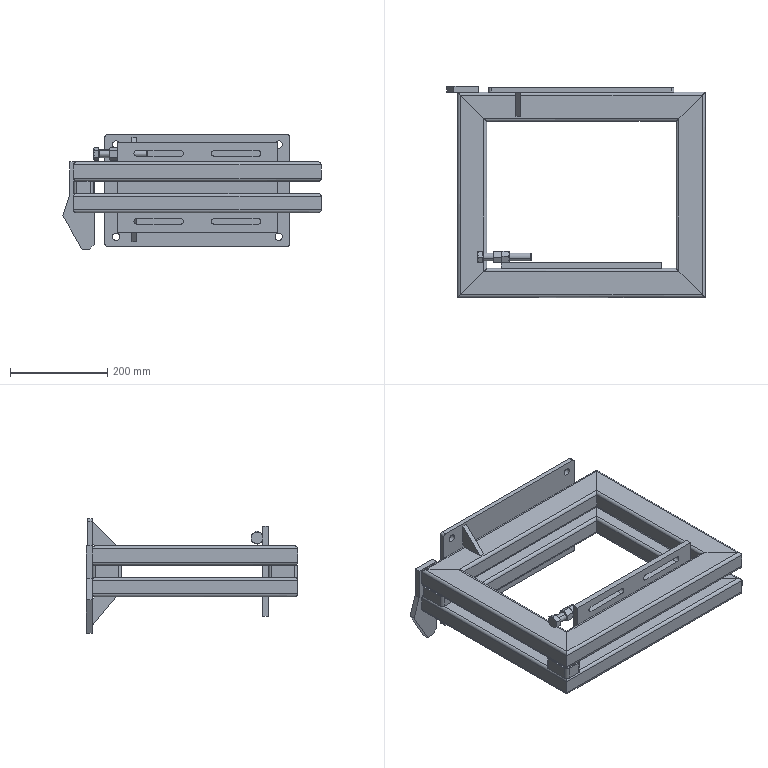Part | SolidWorks | 18 solids | 322 faces | box 532.27 x 435 x 236 mm | volume 3498910 mm3 | plane 166 | cylinder 110 | cone 44 | torus 2 | commonest cylinder face diameters 12 x52 6 x40 15 x8 10 x4 13.835 x4 16 x2